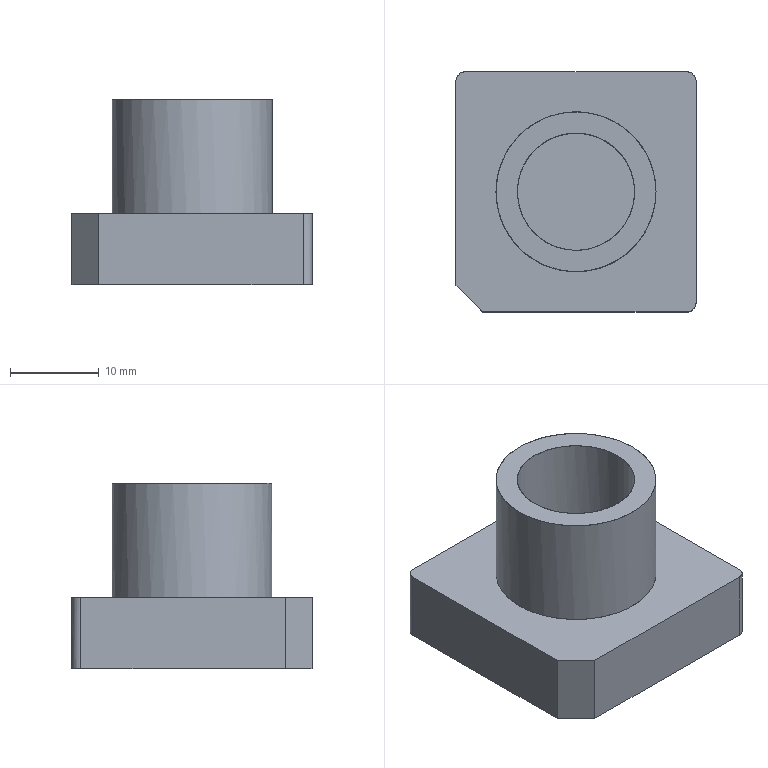CAM job | PowerMill | 3-axis milling, other | part box 27 x 27 x 20.913 mm
Tools:
number,name,type,diameter,tip_radius,length,cutting_length,overhang,flutes,holder,toolpaths_using
1,D10C,end_mill,10.0,0.0,60.0,,30.0,1,D42L35,1
1,D10C_1_1_1,end_mill,10.0,0.0,60.0,,21.36,1,D42L35,3
2,D4C_1_1,end_mill,4.0,0.0,30.0,,13.12,1,D42L35,1
3,D10_1_1_1,end_mill,10.0,0.0,60.0,,21.08,1,D42L35,4
14,D4_1_1,end_mill,4.0,0.0,30.0,,11.84,1,D42L35,2
13,Text_D4_1_1,taper_spherical,4.0,0.3,60.0,,13.16,1,D42L35,1
Operations:
program,toolpath,strategy,tool,tool_number,tool_diameter,tip_radius,flutes,spindle_rpm,feed_cut,surface_speed_m_min_computed,feed_per_tooth_computed,tolerance,thickness,stepover,stepdown,cut_length,cut_time_min,total_time_min,workplane
26-S-0425-3-F,精公开粗01-扫面平行-D10C,raster_area_clear,D10C_1_1_1,1,10.0,0.0,1.0,8000.0,10000.0,251.33,1.25,0.03,0.28,6.0,1.0,260.48,0.026,0.0319,
26-S-0425-3-F,精公开粗01-外形偏置-D10C,offset_area_clear,D10C_1_1_1,1,10.0,0.0,1.0,8000.0,10000.0,251.33,1.25,0.03,0.28,6.0,1.0,7499.281,0.75,0.8329,
26-S-0425-3-F,精公开粗01-基准台等高-D10C,constantz,D10C_1_1_1,1,10.0,0.0,1.0,8000.0,10000.0,251.33,1.25,0.03,0.07,5.0,0.4,3009.073,0.301,0.311,
26-S-0425-3-F,精公再粗02-外形偏置-D4C,offset_area_clear,D4C_1_1,2,4.0,0.0,1.0,18000.0,6000.0,226.19,0.3333,0.03,0.0,2.0,1.0,8094.618,1.349,1.72,
26-S-0425-3-F,精公基准台01-平坦面平行-D10,raster_area_clear,D10_1_1_1,3,10.0,0.0,1.0,8500.0,600.0,267.04,0.0706,0.005,0.38,5.0,1.0,147.865,0.246,0.2628,
26-S-0425-3-F,精公基准台01-基准面偏置-D10,offset_area_clear,D10_1_1_1,3,10.0,0.0,1.0,8500.0,600.0,267.04,0.0706,0.005,0.38,5.0,1.0,100.352,0.167,0.1864,
26-S-0425-3-F,精公基准台01-外形侧光-D10,profile_area_clear,D10_1_1_1,3,10.0,0.0,1.0,8500.0,600.0,267.04,0.0706,0.005,-0.07,0.08,1.0,175.547,0.293,0.3134,
26-S-0425-3-F,精公基准台01-基准台侧光-D10,profile_area_clear,D10_1_1_1,3,10.0,0.0,1.0,8500.0,600.0,267.04,0.0706,0.005,0.0,0.08,1.0,273.233,0.455,0.5201,
26-S-0425-3-F,精公精光01-等高-D4,constantz,D4_1_1,14,4.0,0.0,1.0,18000.0,2000.0,226.19,0.1111,0.005,-0.075,5.0,0.04,8554.046,4.277,4.762,
26-S-0425-3-F,精公精光01-平坦面偏置-D4,offset_area_clear,D4_1_1,14,4.0,0.0,1.0,18000.0,600.0,226.19,0.0333,0.005,0.375,2.0,1.0,160.738,0.268,0.3256,
26-S-0425-3-F,精公刻字01-刻字-Text_D4,pattern,Text_D4_1_1,13,4.0,0.3,1.0,15000.0,1000.0,188.5,0.0667,0.005,0.0,5.0,1.0,46.257,0.046,0.0729,
,精公开粗01-外形偏置-D10C_Reference,offset_area_clear,D10C,1,10.0,0.0,1.0,8000.0,10000.0,251.33,1.25,0.03,0.28,6.0,1.0,14771.296,1.477,1.638,